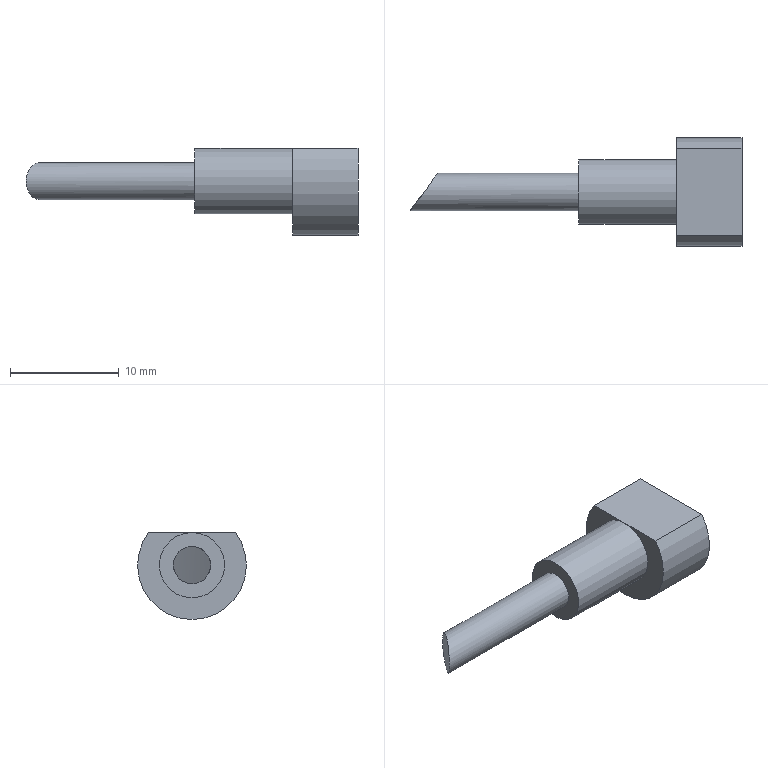Part | NX | features solid 2 | 1 solid | 8 faces | box 30.505 x 10 x 8 mm | volume 788.804 mm3 | plane 4 | cylinder 3 | cone 1 | commonest cylinder face diameters 3.417 x1 6 x1 10 x1
STEP:
#1=CARTESIAN_POINT('',(64.275,-26.15,-8.375));
#2=VERTEX_POINT('',#1);
#3=CARTESIAN_POINT('',(64.275,-34.15,-8.375));
#4=VERTEX_POINT('',#3);
#5=CARTESIAN_POINT('',(64.275,-30.15,-11.375));
#6=DIRECTION('',(-1.,0.,0.));
#7=DIRECTION('',(0.,0.,1.));
#8=AXIS2_PLACEMENT_3D('',#5,#6,#7);
#9=CIRCLE('',#8,5.);
#10=EDGE_CURVE('',#2,#4,#9,.T.);
#11=ORIENTED_EDGE('',*,*,#10,.F.);
#12=CARTESIAN_POINT('',(70.275,-26.15,-8.375));
#13=VERTEX_POINT('',#12);
#14=CARTESIAN_POINT('',(70.275,-26.15,-8.375));
#15=DIRECTION('',(-1.,0.,0.));
#16=VECTOR('',#15,1000.);
#17=LINE('',#14,#16);
#18=EDGE_CURVE('',#2,#13,#17,.F.);
#19=ORIENTED_EDGE('',*,*,#18,.T.);
#20=CARTESIAN_POINT('',(70.275,-34.15,-8.375));
#21=VERTEX_POINT('',#20);
#22=CARTESIAN_POINT('',(70.275,-30.15,-11.375));
#23=DIRECTION('',(-1.,0.,0.));
#24=DIRECTION('',(0.,0.,1.));
#25=AXIS2_PLACEMENT_3D('',#22,#23,#24);
#26=CIRCLE('',#25,5.);
#27=EDGE_CURVE('',#13,#21,#26,.T.);
#28=ORIENTED_EDGE('',*,*,#27,.T.);
#29=CARTESIAN_POINT('',(70.275,-34.15,-8.375));
#30=DIRECTION('',(-1.,0.,0.));
#31=VECTOR('',#30,1000.);
#32=LINE('',#29,#31);
#33=EDGE_CURVE('',#21,#4,#32,.T.);
#34=ORIENTED_EDGE('',*,*,#33,.T.);
#35=EDGE_LOOP('',(#11,#19,#28,#34));
#36=FACE_BOUND('',#35,.T.);
#37=CARTESIAN_POINT('',(70.275,-30.15,-11.375));
#38=DIRECTION('',(-1.,0.,0.));
#39=DIRECTION('',(0.,0.,1.));
#40=AXIS2_PLACEMENT_3D('',#37,#38,#39);
#41=CYLINDRICAL_SURFACE('',#40,5.);
#42=ADVANCED_FACE('',(#36),#41,.T.);
#43=CARTESIAN_POINT('',(64.275,-30.15,-8.375));
#44=VERTEX_POINT('',#43);
#45=CARTESIAN_POINT('',(64.275,-30.15,-11.375));
#46=DIRECTION('',(-1.,0.,0.));
#47=DIRECTION('',(0.,0.,1.));
#48=AXIS2_PLACEMENT_3D('',#45,#46,#47);
#49=CIRCLE('',#48,3.);
#50=EDGE_CURVE('',#44,#44,#49,.T.);
#51=ORIENTED_EDGE('',*,*,#50,.T.);
#52=EDGE_LOOP('',(#51));
#53=FACE_BOUND('',#52,.T.);
#54=CARTESIAN_POINT('',(55.275,-30.15,-14.375));
#55=VERTEX_POINT('',#54);
#56=CARTESIAN_POINT('',(55.275,-30.15,-11.375));
#57=DIRECTION('',(1.,0.,0.));
#58=DIRECTION('',(0.,0.,-1.));
#59=AXIS2_PLACEMENT_3D('',#56,#57,#58);
#60=CIRCLE('',#59,3.);
#61=EDGE_CURVE('',#55,#55,#60,.T.);
#62=ORIENTED_EDGE('',*,*,#61,.T.);
#63=EDGE_LOOP('',(#62));
#64=FACE_BOUND('',#63,.T.);
#65=CARTESIAN_POINT('',(-39.725,-30.15,-11.375));
#66=DIRECTION('',(1.,0.,0.));
#67=DIRECTION('',(0.,0.,-1.));
#68=AXIS2_PLACEMENT_3D('',#65,#66,#67);
#69=CYLINDRICAL_SURFACE('',#68,3.);
#70=ADVANCED_FACE('',(#53,#64),#69,.T.);
#71=CARTESIAN_POINT('',(55.275,-28.442,-11.375));
#72=VERTEX_POINT('',#71);
#73=CARTESIAN_POINT('',(55.275,-30.15,-11.375));
#74=DIRECTION('',(-1.,0.,0.));
#75=DIRECTION('',(0.,1.,0.));
#76=AXIS2_PLACEMENT_3D('',#73,#74,#75);
#77=CIRCLE('',#76,1.708);
#78=EDGE_CURVE('',#72,#72,#77,.T.);
#79=ORIENTED_EDGE('',*,*,#78,.F.);
#80=EDGE_LOOP('',(#79));
#81=FACE_BOUND('',#80,.T.);
#82=ORIENTED_EDGE('',*,*,#61,.F.);
#83=EDGE_LOOP('',(#82));
#84=FACE_BOUND('',#83,.T.);
#85=CARTESIAN_POINT('',(55.275,0.,-24.942));
#86=DIRECTION('',(1.,0.,0.));
#87=DIRECTION('',(0.,0.,-1.));
#88=AXIS2_PLACEMENT_3D('',#85,#86,#87);
#89=PLANE('',#88);
#90=ADVANCED_FACE('',(#81,#84),#89,.F.);
#91=CARTESIAN_POINT('',(39.77,-31.858,-11.374));
#92=VERTEX_POINT('',#91);
#93=CARTESIAN_POINT('',(40.171,-31.378,-9.938));
#94=CARTESIAN_POINT('',(39.576,-32.099,-11.373));
#95=CARTESIAN_POINT('',(40.143,-31.378,-12.815));
#96=CARTESIAN_POINT('',(41.059,-30.169,-13.213));
#97=CARTESIAN_POINT('',(41.936,-28.937,-12.833));
#98=CARTESIAN_POINT('',(42.444,-28.197,-11.389));
#99=CARTESIAN_POINT('',(41.972,-28.925,-9.919));
#100=CARTESIAN_POINT('',(41.086,-30.18,-9.536));
#101=CARTESIAN_POINT('',(40.171,-31.378,-9.938));
#102=CARTESIAN_POINT('',(39.576,-32.099,-11.373));
#103=CARTESIAN_POINT('',(40.143,-31.378,-12.815));
#104=B_SPLINE_CURVE_WITH_KNOTS('',3,(#93,#94,#95,#96,#97,#98,#99,#100,#101,#102,#103),.UNSPECIFIED.,.T.,.F.,(1,1,1,1,1,1,1,1,1,1,1,1,1,1,1),(-0.004498,-0.002998,-0.001499,0.,0.001499,0.002998,0.004498,0.005997,0.007496,0.008995,0.01049,0.01199,0.01349,0.01499,0.01649),.UNSPECIFIED.);
#105=EDGE_CURVE('',#92,#92,#104,.T.);
#106=ORIENTED_EDGE('',*,*,#105,.F.);
#107=EDGE_LOOP('',(#106));
#108=FACE_BOUND('',#107,.T.);
#109=CARTESIAN_POINT('',(0.,0.,-14.088));
#110=DIRECTION('',(0.,0.,1.));
#111=DIRECTION('',(-1.,0.,0.));
#112=AXIS2_PLACEMENT_3D('',#109,#110,#111);
#113=CONICAL_SURFACE('',#112,50.936,0.007653);
#114=ADVANCED_FACE('',(#108),#113,.F.);
#115=ORIENTED_EDGE('',*,*,#105,.T.);
#116=EDGE_LOOP('',(#115));
#117=FACE_BOUND('',#116,.T.);
#118=ORIENTED_EDGE('',*,*,#78,.T.);
#119=EDGE_LOOP('',(#118));
#120=FACE_BOUND('',#119,.T.);
#121=CARTESIAN_POINT('',(55.275,-30.15,-11.375));
#122=DIRECTION('',(1.,0.,0.));
#123=DIRECTION('',(0.,-1.,0.));
#124=AXIS2_PLACEMENT_3D('',#121,#122,#123);
#125=CYLINDRICAL_SURFACE('',#124,1.708);
#126=ADVANCED_FACE('',(#117,#120),#125,.T.);
#127=CARTESIAN_POINT('',(64.275,-30.15,-8.375));
#128=DIRECTION('',(0.,1.,0.));
#129=VECTOR('',#128,1000.);
#130=LINE('',#127,#129);
#131=EDGE_CURVE('',#44,#4,#130,.F.);
#132=ORIENTED_EDGE('',*,*,#131,.F.);
#133=ORIENTED_EDGE('',*,*,#50,.F.);
#134=CARTESIAN_POINT('',(64.275,-30.15,-8.375));
#135=DIRECTION('',(0.,1.,0.));
#136=VECTOR('',#135,1000.);
#137=LINE('',#134,#136);
#138=EDGE_CURVE('',#2,#44,#137,.F.);
#139=ORIENTED_EDGE('',*,*,#138,.F.);
#140=ORIENTED_EDGE('',*,*,#10,.T.);
#141=EDGE_LOOP('',(#132,#133,#139,#140));
#142=FACE_BOUND('',#141,.T.);
#143=CARTESIAN_POINT('',(64.275,-30.15,-11.375));
#144=DIRECTION('',(1.,0.,0.));
#145=DIRECTION('',(0.,0.,-1.));
#146=AXIS2_PLACEMENT_3D('',#143,#144,#145);
#147=PLANE('',#146);
#148=ADVANCED_FACE('',(#142),#147,.F.);
#149=ORIENTED_EDGE('',*,*,#27,.F.);
#150=CARTESIAN_POINT('',(70.275,-30.15,-8.375));
#151=DIRECTION('',(0.,-1.,0.));
#152=VECTOR('',#151,1000.);
#153=LINE('',#150,#152);
#154=EDGE_CURVE('',#13,#21,#153,.T.);
#155=ORIENTED_EDGE('',*,*,#154,.T.);
#156=EDGE_LOOP('',(#149,#155));
#157=FACE_BOUND('',#156,.T.);
#158=CARTESIAN_POINT('',(70.275,0.,3.449));
#159=DIRECTION('',(-1.,0.,0.));
#160=DIRECTION('',(0.,0.,1.));
#161=AXIS2_PLACEMENT_3D('',#158,#159,#160);
#162=PLANE('',#161);
#163=ADVANCED_FACE('',(#157),#162,.F.);
#164=ORIENTED_EDGE('',*,*,#138,.T.);
#165=ORIENTED_EDGE('',*,*,#131,.T.);
#166=ORIENTED_EDGE('',*,*,#33,.F.);
#167=ORIENTED_EDGE('',*,*,#154,.F.);
#168=ORIENTED_EDGE('',*,*,#18,.F.);
#169=EDGE_LOOP('',(#164,#165,#166,#167,#168));
#170=FACE_BOUND('',#169,.T.);
#171=CARTESIAN_POINT('',(67.275,-30.15,-8.375));
#172=DIRECTION('',(0.,0.,1.));
#173=DIRECTION('',(1.,0.,0.));
#174=AXIS2_PLACEMENT_3D('',#171,#172,#173);
#175=PLANE('',#174);
#176=ADVANCED_FACE('',(#170),#175,.T.);
#177=CLOSED_SHELL('',(#42,#70,#90,#114,#126,#148,#163,#176));
#178=MANIFOLD_SOLID_BREP('',#177);
#179=(LENGTH_UNIT()NAMED_UNIT(*)SI_UNIT(.MILLI.,.METRE.));
#180=UNCERTAINTY_MEASURE_WITH_UNIT(LENGTH_MEASURE(0.0508),#179,'','');
#181=(NAMED_UNIT(*)PLANE_ANGLE_UNIT()SI_UNIT($,.RADIAN.));
#182=(NAMED_UNIT(*)SI_UNIT($,.STERADIAN.)SOLID_ANGLE_UNIT());
#183=(GEOMETRIC_REPRESENTATION_CONTEXT(3)GLOBAL_UNCERTAINTY_ASSIGNED_CONTEXT((#180))GLOBAL_UNIT_ASSIGNED_CONTEXT((#179,#181,#182))REPRESENTATION_CONTEXT('',''));
#184=ADVANCED_BREP_SHAPE_REPRESENTATION('',(#178),#183);